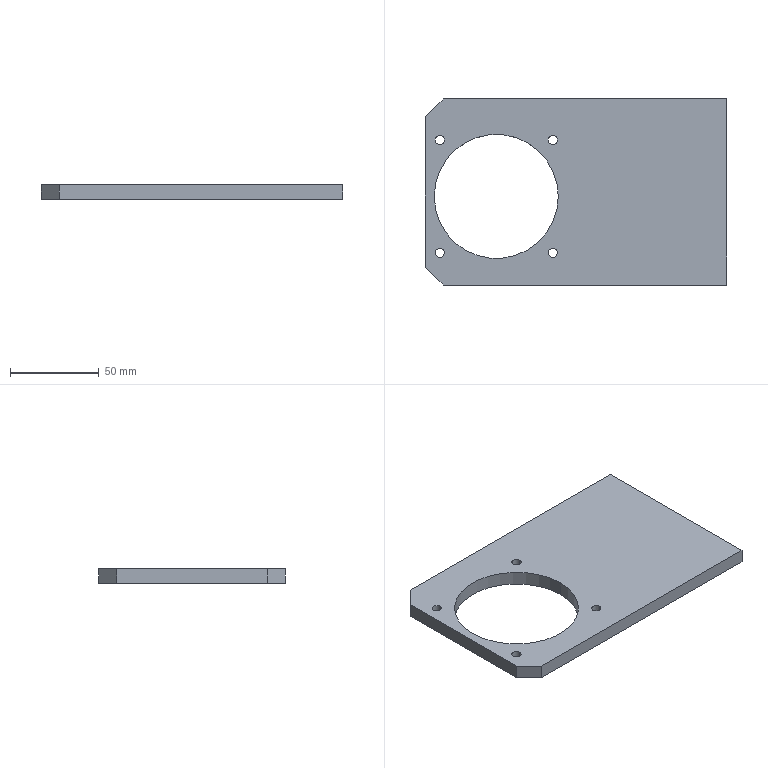Part | STEP file | 1 solid | 18 faces | box 170 x 105 x 8 mm | volume 110533 mm3 | cylinder 10 | plane 8 | commonest cylinder face diameters 5.2 x8 70 x2